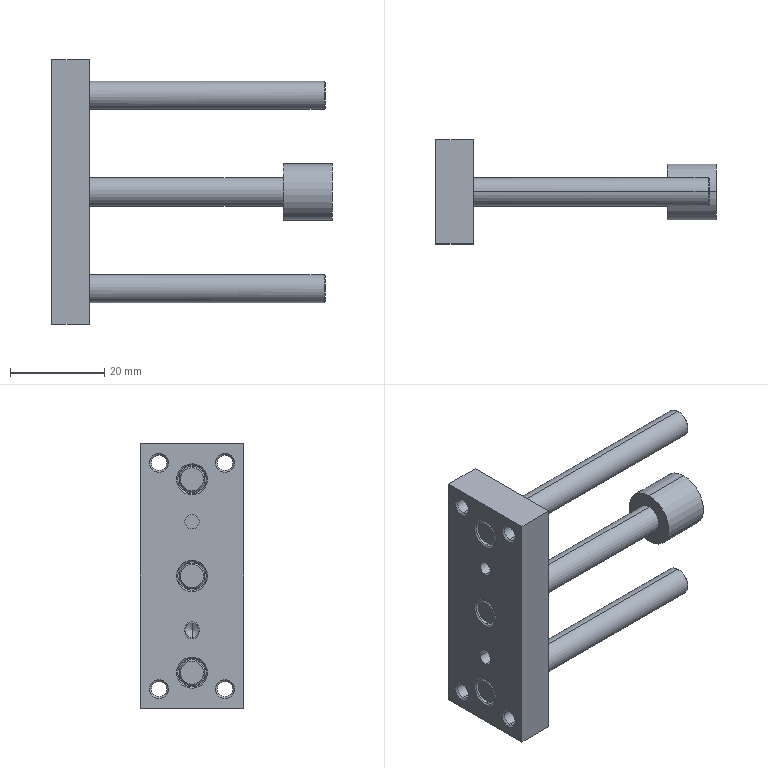Part | SolidWorks | features BaseBody 1 | 1 solid | 90 faces | box 59.5 x 22 x 56 mm | volume 14565 mm3 | cylinder 35 | cone 34 | plane 21 | commonest cylinder face diameters 6 x12 3.242 x8 3 x7 5.5 x6 11.9 x2